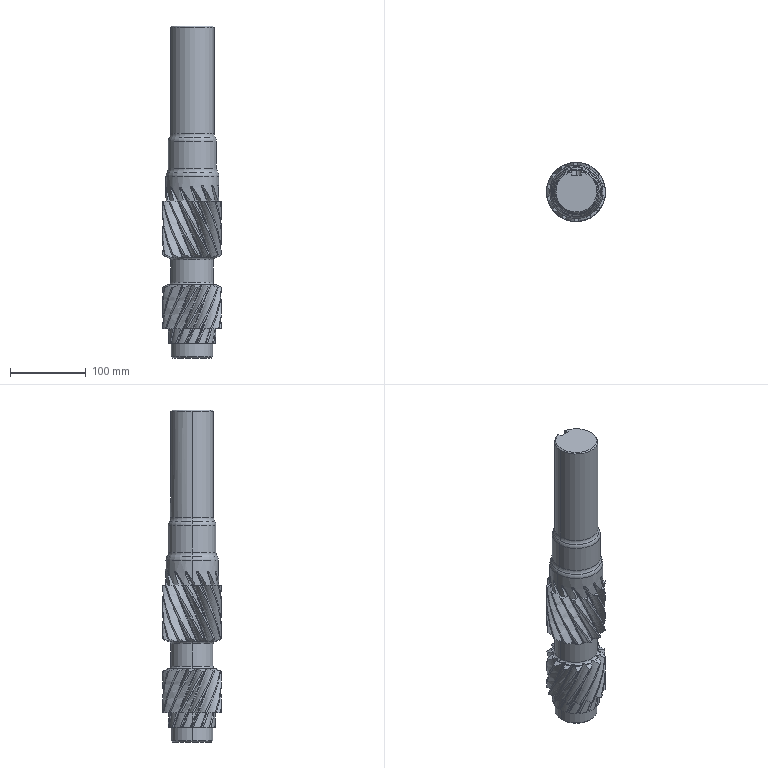Part | SolidWorks | features ICE 5, Chamfer 2, CirPattern 2, Helix 2, SweepCut 2, Extrusion 1, Fillet 1, MirrorSolid 1, RefAxis 1, Revolution 1 | 1 solid | 294 faces | box 77.902 x 77.902 x 438.15 mm | volume 1338068 mm3 | spline 127 | plane 62 | cylinder 58 | cone 35 | torus 12 | commonest cylinder face diameters 77.902 x31 62.23 x15 12.7 x2 55.011 x2 56.312 x2 57.15 x2